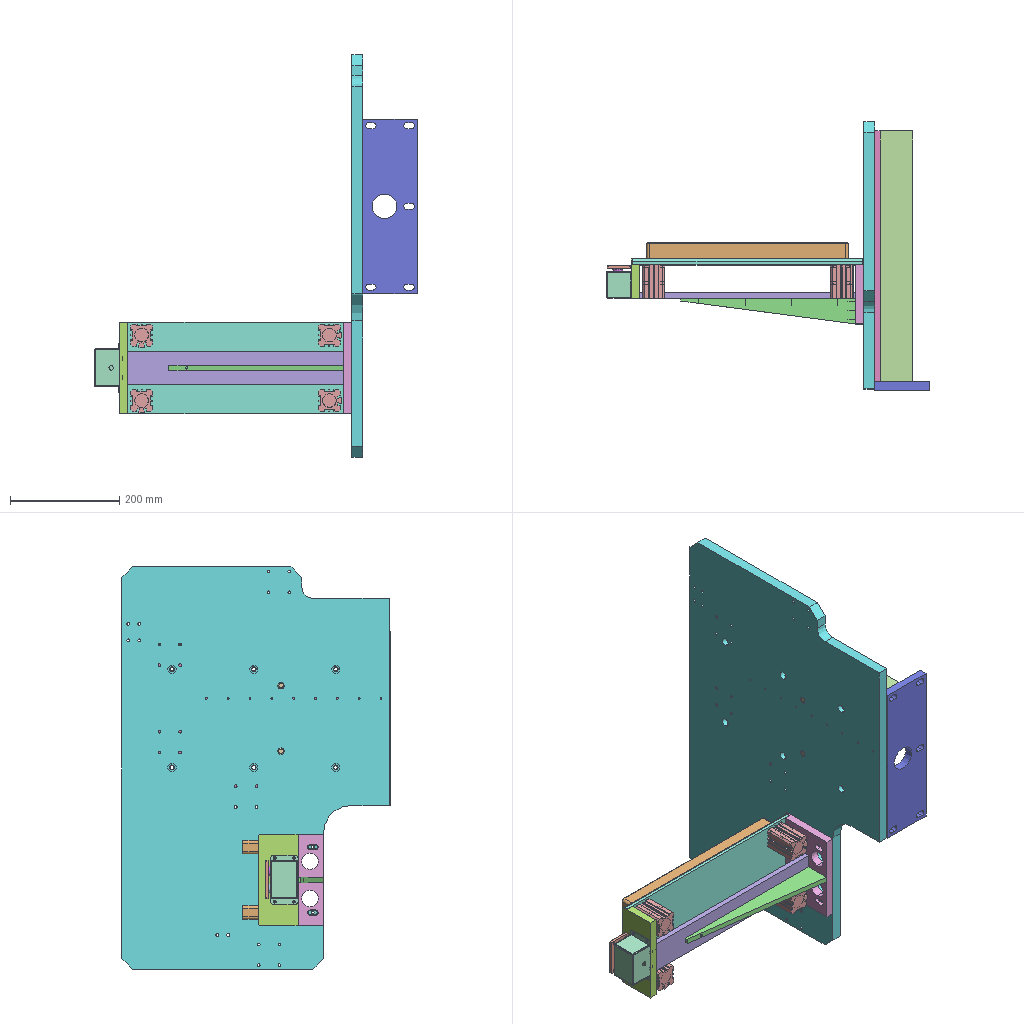Assembly | SolidWorks | 16 different items | 27 placed | box 591 x 492 x 738 mm
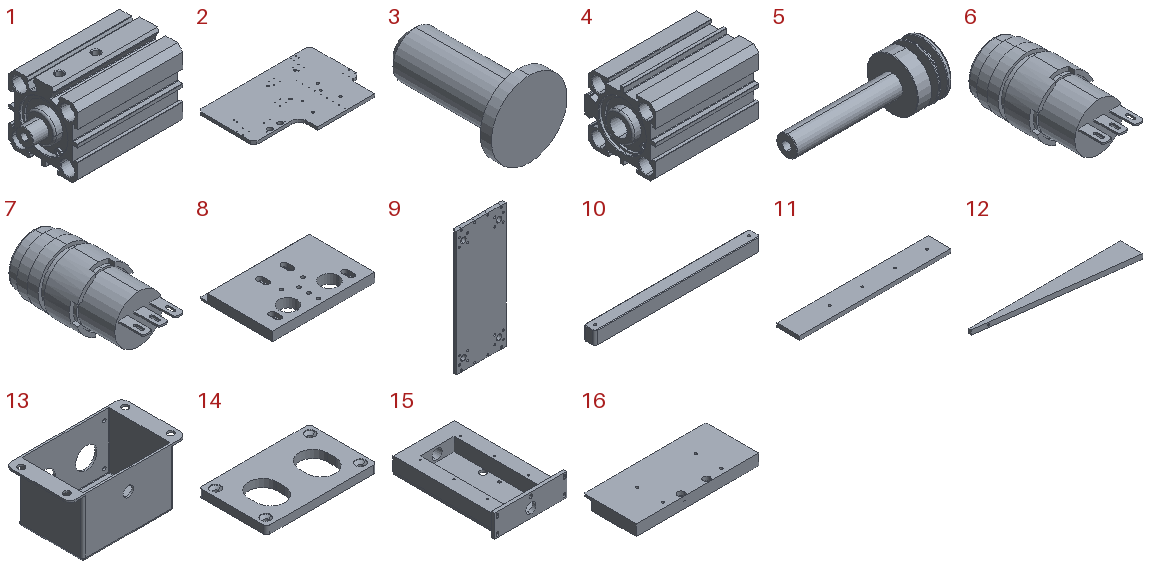Parts list (item | name | quantity | parent item | size | volume | features):
1 | (subassembly) | x4 | - | 72 x 40 x 42 mm | 66610 mm3 | -
2 | - | x1 | - | 738 x 490 x 20 mm | 6263387 mm3 | features HoleWzd 6, Cut 4, Chamfer 2, Extrusion 1
3 | - | x2 | - | 20 x 32 x 20 mm | 4155 mm3 | features Chamfer 1, Revolution 1
4 | - | x4 | in 1 | 63 x 42 x 40 mm | 56645 mm3 | features RefAxis 21, 3DProfileFeature 7, RevCut 6, Extrusion 1, ICE 1, LPattern 1, Revolution 1
5 | - | x4 | in 1 | 68 x 24.9 x 24.9 mm | 9965 mm3 | features RefAxis 6, 3DProfileFeature 2, Revolution 2, HoleWzd 1
6 | - | x1 | - | 18.5 x 41 x 18.5 mm | 7334 mm3 | features ICE 7, Fillet 2, CirPattern 1, Extrusion 1, RevCutThin 1
7 | - | x1 | - | 18.5 x 41 x 18.5 mm | 7334 mm3 | features ICE 7, Fillet 2, CirPattern 1, Extrusion 1, RevCutThin 1
8 | - | x1 | - | 168 x 120 x 15 mm | 244449 mm3 | features HoleWzd 11, Cut 4, ICE 4, Chamfer 1, Extrusion 1, Fillet 1
9 | - | x1 | - | 168 x 12 x 420 mm | 807216 mm3 | features HoleWzd 2, ICE 2, MirrorPattern 2, Extrusion 1, Fillet 1, LPattern 1
10 | - | x2 | - | 370 x 25 x 30 mm | 274027 mm3 | features Chamfer 1, Extrusion 1, Fillet 1, HoleWzd 1
11 | - | x1 | - | 396 x 60 x 10 mm | 234690 mm3 | features HoleWzd 2, Extrusion 1, MirrorPattern 1
12 | - | x1 | - | 320 x 47 x 10 mm | 81873 mm3 | features HoleWzd 2, Extrusion 1
13 | - | x1 | - | 90 x 50 x 45 mm | 20794 mm3 | features ICE 4, Fillet 2, Emboss 1, Extrusion 1, HoleWzd 1, Shell 1
14 | - | x1 | - | 70 x 43 x 5 mm | 11317 mm3 | features Extrusion 1, HoleWzd 1
15 | - | x1 | - | 320 x 475 x 100 mm | 5416407 mm3 | features ICE 4, Cut 3, Extrusion 1, HoleWzd 1
16 | - | x1 | - | 168 x 72 x 15 mm | 156428 mm3 | features HoleWzd 10, ICE 4, Chamfer 2, Cut 1, Extrusion 1, Fillet 1
Mates (type | each side: item.copy, entity, surface, feature):
In the top assembly
Concentric | 5.1 face cylinder Revolve1 | 9.1 face cylinder Mirror2
Concentric | 5.2 face cylinder Revolve1 | 9.1 face cylinder Cut-Extrude1
Coincident | 5.2 face plane Revolve1 | 10.1 face plane Boss-Extrude1
Coincident | 5.3 face plane Revolve1 | 10.1 face plane Boss-Extrude1
Coincident | 5.1 face plane Revolve1 | 10.2 face plane Boss-Extrude1
Coincident | 5.4 face plane Revolve1 | 10.2 face plane Boss-Extrude1
Concentric | 5.3 face cylinder Revolve1 | 9.1 face cylinder Mirror1
Coincident | 4.1 face plane Boss-Extrude1 | 9.1 face plane Boss-Extrude1
Concentric | 5.4 face cylinder Revolve1 | 9.1 face cylinder Mirror2
Coincident | 4.2 face plane Boss-Extrude1 | 9.1 face plane Boss-Extrude1
Parallel | 4.1 face plane Boss-Extrude1 | 9.1 face plane Boss-Extrude1
Coincident | 4.2 face plane Boss-Extrude1 | 4.1 face plane Boss-Extrude1
Parallel | 4.3 face plane Boss-Extrude1 | 9.1 face plane Boss-Extrude1
Coincident | 4.3 face plane Boss-Extrude1 | 4.4 face plane Boss-Extrude1
Coincident | 16.1 face plane Cut-Extrude1 | 9.1 face plane Boss-Extrude1 | 2 times
Coincident | 8.1 face plane Cut-Extrude1 | 9.1 face plane Boss-Extrude1 | 2 times
Concentric | 5.1 face cylinder Revolve1 | 10.2 face cylinder Hole size per socket head cap screw type 1
Concentric | 5.2 face cylinder Revolve1 | 10.1 face cylinder Hole size per socket head cap screw type 1
Coincident | 8.1 face plane Boss-Extrude1 | 9.1 face plane Boss-Extrude1
Concentric | 5.3 face cylinder Revolve1 | 10.1 face cylinder Hole size per socket head cap screw type 1
Concentric | 5.4 face cylinder Revolve1 | 10.2 face cylinder Hole size per socket head cap screw type 1
Coincident | 8.1 face plane Boss-Extrude1 | 11.1 face plane Boss-Extrude1
Width | 8.1 face plane Boss-Extrude1 | 8.1 face plane Boss-Extrude1 | 11.1 face plane Boss-Extrude1 | 11.1 face plane Boss-Extrude1
Coincident | 16.1 face plane Cut-Extrude6 | 11.1 face plane Boss-Extrude1
Coincident | 8.1 face plane Boss-Extrude1 | 12.1 face plane Boss-Extrude1
Coincident | 11.1 face plane Boss-Extrude1 | 12.1 face plane Boss-Extrude1
Width | 11.1 face plane Boss-Extrude1 | 11.1 face plane Boss-Extrude1 | 12.1 face plane Boss-Extrude1 | 12.1 face plane Boss-Extrude1
Coincident | 7.1 face plane Boss-Extrude4 | 6.1 face plane Boss-Extrude4
Coincident | 7.1 face plane Boss-Extrude5 | 6.1 face plane Boss-Extrude5
Concentric | 7.1 face cylinder Boss-Extrude2 | 13.1 face cylinder Cut-Extrude2
Coincident | 6.1 face plane Boss-Extrude1 | 13.1 face plane Boss-Extrude1
Concentric | 6.1 face cylinder Boss-Extrude2 | 13.1 face cylinder Cut-Extrude2
Parallel | 6.1 face plane Boss-Extrude5 | 13.1 face plane Boss-Extrude1
DistanceDim | 14.1 face plane Boss-Extrude1 | 13.1 face plane Boss-Extrude1
Concentric | 14.1 face cylinder CSK for M3 Flat Head Machine Screw1 | 13.1 face cylinder M3 Tapped Hole1
Concentric | 13.1 face cylinder M3 Tapped Hole1 | 14.1 face cylinder CSK for M3 Flat Head Machine Screw1
Coincident | 2.1 face plane Boss-Extrude3 | 8.1 face plane Boss-Extrude1
DistanceDim | 9.1 face plane Boss-Extrude1 | 2.1 face plane Boss-Extrude3
Coincident | 2.1 face plane Boss-Extrude3 | 8.1 face plane Cut-Extrude6
Coincident | 2.1 face plane Boss-Extrude3 | 15.1 face plane Boss-Extrude3
Coincident | 15.1 face plane Boss-Extrude4 | 2.1 face plane Boss-Extrude3
Width | 16.1 face plane Boss-Extrude1 | 16.1 face plane Boss-Extrude1 | 9.1 face plane Boss-Extrude1 | 9.1 face plane Boss-Extrude1
Concentric | 16.1 face cylinder M4 Tapped Hole2 | 13.1 face cylinder Cut-Extrude1 | 2 times
Coincident | 16.1 face plane Boss-Extrude1 | 13.1 face plane Boss-Extrude1
DistanceDim | 2.1 face plane Boss-Extrude3 | 15.1 face plane Boss-Extrude4
Coincident | 15.1 face plane Boss-Extrude3 | 3.1 face plane Revolve1
Concentric | 15.1 face cylinder Cut-Extrude6 | 3.1 face cylinder Revolve1
Coincident | 3.1 face plane Revolve1 | 3.2 face plane Revolve1
Concentric | 15.1 face cylinder Cut-Extrude6 | 3.2 face cylinder Revolve1
In subassembly 1
Coincident | 4.5 axis | 5.5 axis | 2 times
PlanarAngleDim | 5.5 plane | 4.5 plane
LimitDistanceDim | 5.5 face plane Revolve2 | 4.5 face plane Cut-Revolve4